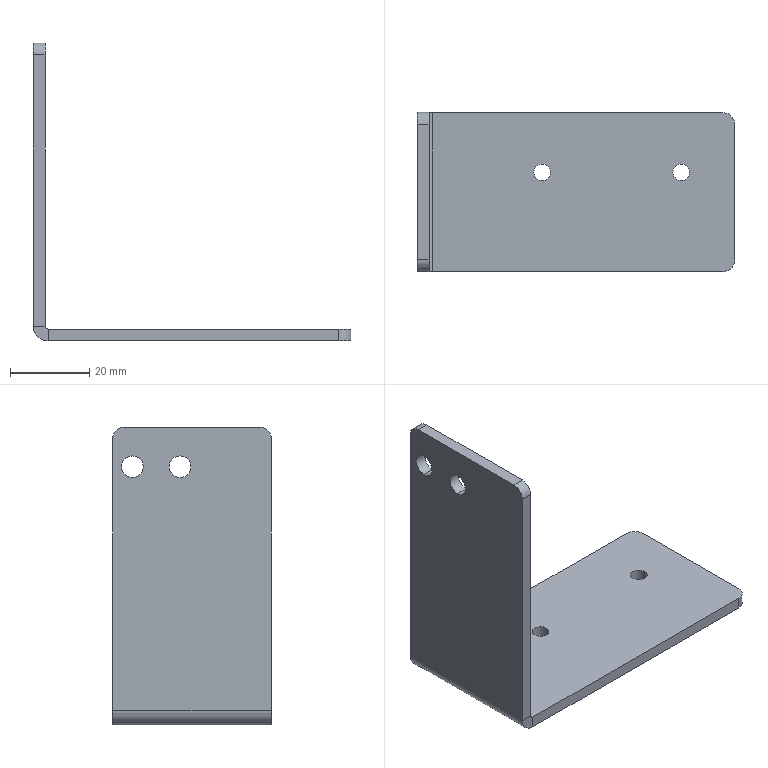Part | SolidWorks | features HoleWzd 2, Fillet 1, FlatPattern 1, SMBaseFlange 1, SheetMetal 1 | 1 solid | 26 faces | box 80 x 40 x 75 mm | volume 17875 mm3 | cylinder 14 | plane 12 | commonest cylinder face diameters 4.2 x4 5.5 x4 6 x4 1.5 x1 7.5 x1
STEP:
#1=CARTESIAN_POINT('',(3.,35.,-12.75));
#2=VERTEX_POINT('',#1);
#3=CARTESIAN_POINT('',(3.,35.,-7.25));
#4=VERTEX_POINT('',#3);
#5=CARTESIAN_POINT('',(3.,35.,-10.));
#6=DIRECTION('',(-1.,0.,0.));
#7=DIRECTION('',(0.,0.,1.));
#8=AXIS2_PLACEMENT_3D('',#5,#6,#7);
#9=CIRCLE('',#8,2.75);
#10=EDGE_CURVE('',#2,#4,#9,.T.);
#11=ORIENTED_EDGE('',*,*,#10,.F.);
#12=CARTESIAN_POINT('',(0.,35.,-12.75));
#13=VERTEX_POINT('',#12);
#14=CARTESIAN_POINT('',(0.,35.,-12.75));
#15=DIRECTION('',(-1.,0.,0.));
#16=VECTOR('',#15,1000.);
#17=LINE('',#14,#16);
#18=EDGE_CURVE('',#2,#13,#17,.T.);
#19=ORIENTED_EDGE('',*,*,#18,.T.);
#20=CARTESIAN_POINT('',(0.,35.,-7.25));
#21=VERTEX_POINT('',#20);
#22=CARTESIAN_POINT('',(0.,35.,-10.));
#23=DIRECTION('',(-1.,0.,0.));
#24=DIRECTION('',(0.,0.,1.));
#25=AXIS2_PLACEMENT_3D('',#22,#23,#24);
#26=CIRCLE('',#25,2.75);
#27=EDGE_CURVE('',#13,#21,#26,.T.);
#28=ORIENTED_EDGE('',*,*,#27,.T.);
#29=CARTESIAN_POINT('',(0.,35.,-7.25));
#30=DIRECTION('',(-1.,0.,0.));
#31=VECTOR('',#30,1000.);
#32=LINE('',#29,#31);
#33=EDGE_CURVE('',#4,#21,#32,.T.);
#34=ORIENTED_EDGE('',*,*,#33,.F.);
#35=EDGE_LOOP('',(#11,#19,#28,#34));
#36=FACE_OUTER_BOUND('',#35,.T.);
#37=CARTESIAN_POINT('',(0.,35.,-10.));
#38=DIRECTION('',(-1.,0.,0.));
#39=DIRECTION('',(0.,0.,1.));
#40=AXIS2_PLACEMENT_3D('',#37,#38,#39);
#41=CYLINDRICAL_SURFACE('',#40,2.75);
#42=ADVANCED_FACE('',(#36),#41,.F.);
#43=CARTESIAN_POINT('',(3.,23.,-12.75));
#44=VERTEX_POINT('',#43);
#45=CARTESIAN_POINT('',(3.,23.,-7.25));
#46=VERTEX_POINT('',#45);
#47=CARTESIAN_POINT('',(3.,23.,-10.));
#48=DIRECTION('',(-1.,0.,0.));
#49=DIRECTION('',(0.,0.,1.));
#50=AXIS2_PLACEMENT_3D('',#47,#48,#49);
#51=CIRCLE('',#50,2.75);
#52=EDGE_CURVE('',#44,#46,#51,.T.);
#53=ORIENTED_EDGE('',*,*,#52,.F.);
#54=CARTESIAN_POINT('',(0.,23.,-12.75));
#55=VERTEX_POINT('',#54);
#56=CARTESIAN_POINT('',(0.,23.,-12.75));
#57=DIRECTION('',(-1.,0.,0.));
#58=VECTOR('',#57,1000.);
#59=LINE('',#56,#58);
#60=EDGE_CURVE('',#44,#55,#59,.T.);
#61=ORIENTED_EDGE('',*,*,#60,.T.);
#62=CARTESIAN_POINT('',(0.,23.,-7.25));
#63=VERTEX_POINT('',#62);
#64=CARTESIAN_POINT('',(0.,23.,-10.));
#65=DIRECTION('',(-1.,0.,0.));
#66=DIRECTION('',(0.,0.,1.));
#67=AXIS2_PLACEMENT_3D('',#64,#65,#66);
#68=CIRCLE('',#67,2.75);
#69=EDGE_CURVE('',#55,#63,#68,.T.);
#70=ORIENTED_EDGE('',*,*,#69,.T.);
#71=CARTESIAN_POINT('',(0.,23.,-7.25));
#72=DIRECTION('',(-1.,0.,0.));
#73=VECTOR('',#72,1000.);
#74=LINE('',#71,#73);
#75=EDGE_CURVE('',#46,#63,#74,.T.);
#76=ORIENTED_EDGE('',*,*,#75,.F.);
#77=EDGE_LOOP('',(#53,#61,#70,#76));
#78=FACE_OUTER_BOUND('',#77,.T.);
#79=CARTESIAN_POINT('',(0.,23.,-10.));
#80=DIRECTION('',(-1.,0.,0.));
#81=DIRECTION('',(0.,0.,1.));
#82=AXIS2_PLACEMENT_3D('',#79,#80,#81);
#83=CYLINDRICAL_SURFACE('',#82,2.75);
#84=ADVANCED_FACE('',(#78),#83,.F.);
#85=CARTESIAN_POINT('',(68.6,25.,-72.));
#86=VERTEX_POINT('',#85);
#87=CARTESIAN_POINT('',(64.4,25.,-72.));
#88=VERTEX_POINT('',#87);
#89=CARTESIAN_POINT('',(66.5,25.,-72.));
#90=DIRECTION('',(0.,0.,-1.));
#91=DIRECTION('',(-1.,0.,0.));
#92=AXIS2_PLACEMENT_3D('',#89,#90,#91);
#93=CIRCLE('',#92,2.1);
#94=EDGE_CURVE('',#86,#88,#93,.T.);
#95=ORIENTED_EDGE('',*,*,#94,.F.);
#96=CARTESIAN_POINT('',(68.6,25.,-75.));
#97=VERTEX_POINT('',#96);
#98=CARTESIAN_POINT('',(68.6,25.,-75.));
#99=DIRECTION('',(0.,0.,-1.));
#100=VECTOR('',#99,1000.);
#101=LINE('',#98,#100);
#102=EDGE_CURVE('',#86,#97,#101,.T.);
#103=ORIENTED_EDGE('',*,*,#102,.T.);
#104=CARTESIAN_POINT('',(64.4,25.,-75.));
#105=VERTEX_POINT('',#104);
#106=CARTESIAN_POINT('',(66.5,25.,-75.));
#107=DIRECTION('',(0.,0.,-1.));
#108=DIRECTION('',(-1.,0.,0.));
#109=AXIS2_PLACEMENT_3D('',#106,#107,#108);
#110=CIRCLE('',#109,2.1);
#111=EDGE_CURVE('',#97,#105,#110,.T.);
#112=ORIENTED_EDGE('',*,*,#111,.T.);
#113=CARTESIAN_POINT('',(64.4,25.,-75.));
#114=DIRECTION('',(0.,0.,-1.));
#115=VECTOR('',#114,1000.);
#116=LINE('',#113,#115);
#117=EDGE_CURVE('',#88,#105,#116,.T.);
#118=ORIENTED_EDGE('',*,*,#117,.F.);
#119=EDGE_LOOP('',(#95,#103,#112,#118));
#120=FACE_OUTER_BOUND('',#119,.T.);
#121=CARTESIAN_POINT('',(66.5,25.,-75.));
#122=DIRECTION('',(0.,0.,-1.));
#123=DIRECTION('',(-1.,0.,0.));
#124=AXIS2_PLACEMENT_3D('',#121,#122,#123);
#125=CYLINDRICAL_SURFACE('',#124,2.1);
#126=ADVANCED_FACE('',(#120),#125,.F.);
#127=CARTESIAN_POINT('',(33.6,25.,-72.));
#128=VERTEX_POINT('',#127);
#129=CARTESIAN_POINT('',(29.4,25.,-72.));
#130=VERTEX_POINT('',#129);
#131=CARTESIAN_POINT('',(31.5,25.,-72.));
#132=DIRECTION('',(0.,0.,-1.));
#133=DIRECTION('',(-1.,0.,0.));
#134=AXIS2_PLACEMENT_3D('',#131,#132,#133);
#135=CIRCLE('',#134,2.1);
#136=EDGE_CURVE('',#128,#130,#135,.T.);
#137=ORIENTED_EDGE('',*,*,#136,.F.);
#138=CARTESIAN_POINT('',(33.6,25.,-75.));
#139=VERTEX_POINT('',#138);
#140=CARTESIAN_POINT('',(33.6,25.,-75.));
#141=DIRECTION('',(0.,0.,-1.));
#142=VECTOR('',#141,1000.);
#143=LINE('',#140,#142);
#144=EDGE_CURVE('',#128,#139,#143,.T.);
#145=ORIENTED_EDGE('',*,*,#144,.T.);
#146=CARTESIAN_POINT('',(29.4,25.,-75.));
#147=VERTEX_POINT('',#146);
#148=CARTESIAN_POINT('',(31.5,25.,-75.));
#149=DIRECTION('',(0.,0.,-1.));
#150=DIRECTION('',(-1.,0.,0.));
#151=AXIS2_PLACEMENT_3D('',#148,#149,#150);
#152=CIRCLE('',#151,2.1);
#153=EDGE_CURVE('',#139,#147,#152,.T.);
#154=ORIENTED_EDGE('',*,*,#153,.T.);
#155=CARTESIAN_POINT('',(29.4,25.,-75.));
#156=DIRECTION('',(0.,0.,-1.));
#157=VECTOR('',#156,1000.);
#158=LINE('',#155,#157);
#159=EDGE_CURVE('',#130,#147,#158,.T.);
#160=ORIENTED_EDGE('',*,*,#159,.F.);
#161=EDGE_LOOP('',(#137,#145,#154,#160));
#162=FACE_OUTER_BOUND('',#161,.T.);
#163=CARTESIAN_POINT('',(31.5,25.,-75.));
#164=DIRECTION('',(0.,0.,-1.));
#165=DIRECTION('',(-1.,0.,0.));
#166=AXIS2_PLACEMENT_3D('',#163,#164,#165);
#167=CYLINDRICAL_SURFACE('',#166,2.1);
#168=ADVANCED_FACE('',(#162),#167,.F.);
#169=CARTESIAN_POINT('',(3.75,40.,-75.));
#170=VERTEX_POINT('',#169);
#171=CARTESIAN_POINT('',(3.75,40.,-72.));
#172=VERTEX_POINT('',#171);
#173=CARTESIAN_POINT('',(3.75,40.,-75.));
#174=DIRECTION('',(0.,0.,1.));
#175=VECTOR('',#174,1000.);
#176=LINE('',#173,#175);
#177=EDGE_CURVE('',#170,#172,#176,.T.);
#178=ORIENTED_EDGE('',*,*,#177,.F.);
#179=CARTESIAN_POINT('',(0.,40.,-71.25));
#180=VERTEX_POINT('',#179);
#181=CARTESIAN_POINT('',(3.75,40.,-71.25));
#182=DIRECTION('',(0.,-1.,0.));
#183=DIRECTION('',(0.,0.,1.));
#184=AXIS2_PLACEMENT_3D('',#181,#182,#183);
#185=CIRCLE('',#184,3.75);
#186=EDGE_CURVE('',#180,#170,#185,.T.);
#187=ORIENTED_EDGE('',*,*,#186,.F.);
#188=CARTESIAN_POINT('',(3.,40.,-71.25));
#189=VERTEX_POINT('',#188);
#190=CARTESIAN_POINT('',(3.,40.,-71.25));
#191=DIRECTION('',(-1.,0.,0.));
#192=VECTOR('',#191,1000.);
#193=LINE('',#190,#192);
#194=EDGE_CURVE('',#189,#180,#193,.T.);
#195=ORIENTED_EDGE('',*,*,#194,.F.);
#196=CARTESIAN_POINT('',(3.75,40.,-71.25));
#197=DIRECTION('',(0.,-1.,0.));
#198=DIRECTION('',(1.,0.,0.));
#199=AXIS2_PLACEMENT_3D('',#196,#197,#198);
#200=CIRCLE('',#199,0.75);
#201=EDGE_CURVE('',#189,#172,#200,.T.);
#202=ORIENTED_EDGE('',*,*,#201,.T.);
#203=EDGE_LOOP('',(#178,#187,#195,#202));
#204=FACE_OUTER_BOUND('',#203,.T.);
#205=CARTESIAN_POINT('',(3.75,40.,-75.));
#206=DIRECTION('',(0.,1.,0.));
#207=DIRECTION('',(0.,0.,1.));
#208=AXIS2_PLACEMENT_3D('',#205,#206,#207);
#209=PLANE('',#208);
#210=ADVANCED_FACE('',(#204),#209,.T.);
#211=CARTESIAN_POINT('',(77.,40.,-72.));
#212=VERTEX_POINT('',#211);
#213=CARTESIAN_POINT('',(0.,40.,-72.));
#214=DIRECTION('',(1.,0.,0.));
#215=VECTOR('',#214,1000.);
#216=LINE('',#213,#215);
#217=EDGE_CURVE('',#172,#212,#216,.T.);
#218=ORIENTED_EDGE('',*,*,#217,.T.);
#219=CARTESIAN_POINT('',(77.,40.,-75.));
#220=VERTEX_POINT('',#219);
#221=CARTESIAN_POINT('',(77.,40.,-71.25));
#222=DIRECTION('',(0.,0.,-1.));
#223=VECTOR('',#222,1000.);
#224=LINE('',#221,#223);
#225=EDGE_CURVE('',#212,#220,#224,.T.);
#226=ORIENTED_EDGE('',*,*,#225,.T.);
#227=CARTESIAN_POINT('',(0.,40.,-75.));
#228=DIRECTION('',(1.,0.,0.));
#229=VECTOR('',#228,1000.);
#230=LINE('',#227,#229);
#231=EDGE_CURVE('',#170,#220,#230,.T.);
#232=ORIENTED_EDGE('',*,*,#231,.F.);
#233=ORIENTED_EDGE('',*,*,#177,.T.);
#234=EDGE_LOOP('',(#218,#226,#232,#233));
#235=FACE_OUTER_BOUND('',#234,.T.);
#236=CARTESIAN_POINT('',(3.,40.,-71.25));
#237=DIRECTION('',(0.,1.,0.));
#238=DIRECTION('',(0.,0.,1.));
#239=AXIS2_PLACEMENT_3D('',#236,#237,#238);
#240=PLANE('',#239);
#241=ADVANCED_FACE('',(#235),#240,.T.);
#242=CARTESIAN_POINT('',(0.,0.,-71.25));
#243=VERTEX_POINT('',#242);
#244=CARTESIAN_POINT('',(3.,0.,-71.25));
#245=VERTEX_POINT('',#244);
#246=CARTESIAN_POINT('',(0.,0.,-71.25));
#247=DIRECTION('',(1.,0.,0.));
#248=VECTOR('',#247,1000.);
#249=LINE('',#246,#248);
#250=EDGE_CURVE('',#243,#245,#249,.T.);
#251=ORIENTED_EDGE('',*,*,#250,.F.);
#252=CARTESIAN_POINT('',(3.75,0.,-75.));
#253=VERTEX_POINT('',#252);
#254=CARTESIAN_POINT('',(3.75,0.,-71.25));
#255=DIRECTION('',(0.,-1.,0.));
#256=DIRECTION('',(0.,0.,1.));
#257=AXIS2_PLACEMENT_3D('',#254,#255,#256);
#258=CIRCLE('',#257,3.75);
#259=EDGE_CURVE('',#243,#253,#258,.T.);
#260=ORIENTED_EDGE('',*,*,#259,.T.);
#261=CARTESIAN_POINT('',(3.75,0.,-72.));
#262=VERTEX_POINT('',#261);
#263=CARTESIAN_POINT('',(3.75,0.,-72.));
#264=DIRECTION('',(0.,0.,-1.));
#265=VECTOR('',#264,1000.);
#266=LINE('',#263,#265);
#267=EDGE_CURVE('',#262,#253,#266,.T.);
#268=ORIENTED_EDGE('',*,*,#267,.F.);
#269=CARTESIAN_POINT('',(3.75,0.,-71.25));
#270=DIRECTION('',(0.,-1.,0.));
#271=DIRECTION('',(1.,0.,0.));
#272=AXIS2_PLACEMENT_3D('',#269,#270,#271);
#273=CIRCLE('',#272,0.75);
#274=EDGE_CURVE('',#245,#262,#273,.T.);
#275=ORIENTED_EDGE('',*,*,#274,.F.);
#276=EDGE_LOOP('',(#251,#260,#268,#275));
#277=FACE_OUTER_BOUND('',#276,.T.);
#278=CARTESIAN_POINT('',(0.,0.,-71.25));
#279=DIRECTION('',(0.,-1.,0.));
#280=DIRECTION('',(0.,0.,-1.));
#281=AXIS2_PLACEMENT_3D('',#278,#279,#280);
#282=PLANE('',#281);
#283=ADVANCED_FACE('',(#277),#282,.T.);
#284=CARTESIAN_POINT('',(3.,0.,-3.));
#285=VERTEX_POINT('',#284);
#286=CARTESIAN_POINT('',(3.,0.,0.));
#287=DIRECTION('',(0.,0.,-1.));
#288=VECTOR('',#287,1000.);
#289=LINE('',#286,#288);
#290=EDGE_CURVE('',#285,#245,#289,.T.);
#291=ORIENTED_EDGE('',*,*,#290,.F.);
#292=CARTESIAN_POINT('',(0.,0.,-3.));
#293=VERTEX_POINT('',#292);
#294=CARTESIAN_POINT('',(3.75,0.,-3.));
#295=DIRECTION('',(-1.,0.,0.));
#296=VECTOR('',#295,1000.);
#297=LINE('',#294,#296);
#298=EDGE_CURVE('',#285,#293,#297,.T.);
#299=ORIENTED_EDGE('',*,*,#298,.T.);
#300=CARTESIAN_POINT('',(0.,0.,0.));
#301=DIRECTION('',(0.,0.,-1.));
#302=VECTOR('',#301,1000.);
#303=LINE('',#300,#302);
#304=EDGE_CURVE('',#293,#243,#303,.T.);
#305=ORIENTED_EDGE('',*,*,#304,.T.);
#306=ORIENTED_EDGE('',*,*,#250,.T.);
#307=EDGE_LOOP('',(#291,#299,#305,#306));
#308=FACE_OUTER_BOUND('',#307,.T.);
#309=CARTESIAN_POINT('',(3.75,0.,-72.));
#310=DIRECTION('',(0.,-1.,0.));
#311=DIRECTION('',(0.,0.,-1.));
#312=AXIS2_PLACEMENT_3D('',#309,#310,#311);
#313=PLANE('',#312);
#314=ADVANCED_FACE('',(#308),#313,.T.);
#315=CARTESIAN_POINT('',(66.5,25.,-72.));
#316=DIRECTION('',(0.,0.,-1.));
#317=DIRECTION('',(-1.,0.,0.));
#318=AXIS2_PLACEMENT_3D('',#315,#316,#317);
#319=CIRCLE('',#318,2.1);
#320=EDGE_CURVE('',#88,#86,#319,.T.);
#321=ORIENTED_EDGE('',*,*,#320,.T.);
#322=ORIENTED_EDGE('',*,*,#94,.T.);
#323=EDGE_LOOP('',(#321,#322));
#324=FACE_BOUND('',#323,.T.);
#325=CARTESIAN_POINT('',(31.5,25.,-72.));
#326=DIRECTION('',(0.,0.,-1.));
#327=DIRECTION('',(-1.,0.,0.));
#328=AXIS2_PLACEMENT_3D('',#325,#326,#327);
#329=CIRCLE('',#328,2.1);
#330=EDGE_CURVE('',#130,#128,#329,.T.);
#331=ORIENTED_EDGE('',*,*,#330,.T.);
#332=ORIENTED_EDGE('',*,*,#136,.T.);
#333=EDGE_LOOP('',(#331,#332));
#334=FACE_BOUND('',#333,.T.);
#335=CARTESIAN_POINT('',(80.,37.,-72.));
#336=VERTEX_POINT('',#335);
#337=CARTESIAN_POINT('',(80.,3.,-72.));
#338=VERTEX_POINT('',#337);
#339=CARTESIAN_POINT('',(80.,40.,-72.));
#340=DIRECTION('',(0.,-1.,0.));
#341=VECTOR('',#340,1000.);
#342=LINE('',#339,#341);
#343=EDGE_CURVE('',#336,#338,#342,.T.);
#344=ORIENTED_EDGE('',*,*,#343,.F.);
#345=CARTESIAN_POINT('',(77.,37.,-72.));
#346=DIRECTION('',(0.,0.,1.));
#347=DIRECTION('',(-1.,0.,0.));
#348=AXIS2_PLACEMENT_3D('',#345,#346,#347);
#349=CIRCLE('',#348,3.);
#350=EDGE_CURVE('',#336,#212,#349,.T.);
#351=ORIENTED_EDGE('',*,*,#350,.T.);
#352=ORIENTED_EDGE('',*,*,#217,.F.);
#353=CARTESIAN_POINT('',(3.75,40.,-72.));
#354=DIRECTION('',(0.,-1.,0.));
#355=VECTOR('',#354,1000.);
#356=LINE('',#353,#355);
#357=EDGE_CURVE('',#172,#262,#356,.T.);
#358=ORIENTED_EDGE('',*,*,#357,.T.);
#359=CARTESIAN_POINT('',(77.,0.,-72.));
#360=VERTEX_POINT('',#359);
#361=CARTESIAN_POINT('',(0.,0.,-72.));
#362=DIRECTION('',(1.,0.,0.));
#363=VECTOR('',#362,1000.);
#364=LINE('',#361,#363);
#365=EDGE_CURVE('',#262,#360,#364,.T.);
#366=ORIENTED_EDGE('',*,*,#365,.T.);
#367=CARTESIAN_POINT('',(77.,3.,-72.));
#368=DIRECTION('',(0.,0.,1.));
#369=DIRECTION('',(-1.,0.,0.));
#370=AXIS2_PLACEMENT_3D('',#367,#368,#369);
#371=CIRCLE('',#370,3.);
#372=EDGE_CURVE('',#360,#338,#371,.T.);
#373=ORIENTED_EDGE('',*,*,#372,.T.);
#374=EDGE_LOOP('',(#344,#351,#352,#358,#366,#373));
#375=FACE_OUTER_BOUND('',#374,.T.);
#376=CARTESIAN_POINT('',(0.,40.,-72.));
#377=DIRECTION('',(0.,0.,-1.));
#378=DIRECTION('',(-1.,0.,0.));
#379=AXIS2_PLACEMENT_3D('',#376,#377,#378);
#380=PLANE('',#379);
#381=ADVANCED_FACE('',(#324,#334,#375),#380,.F.);
#382=CARTESIAN_POINT('',(80.,37.,-75.));
#383=VERTEX_POINT('',#382);
#384=CARTESIAN_POINT('',(80.,3.,-75.));
#385=VERTEX_POINT('',#384);
#386=CARTESIAN_POINT('',(80.,40.,-75.));
#387=DIRECTION('',(0.,-1.,0.));
#388=VECTOR('',#387,1000.);
#389=LINE('',#386,#388);
#390=EDGE_CURVE('',#383,#385,#389,.T.);
#391=ORIENTED_EDGE('',*,*,#390,.F.);
#392=CARTESIAN_POINT('',(80.,37.,-75.));
#393=DIRECTION('',(0.,0.,1.));
#394=VECTOR('',#393,1000.);
#395=LINE('',#392,#394);
#396=EDGE_CURVE('',#383,#336,#395,.T.);
#397=ORIENTED_EDGE('',*,*,#396,.T.);
#398=ORIENTED_EDGE('',*,*,#343,.T.);
#399=CARTESIAN_POINT('',(80.,3.,-75.));
#400=DIRECTION('',(0.,0.,-1.));
#401=VECTOR('',#400,1000.);
#402=LINE('',#399,#401);
#403=EDGE_CURVE('',#338,#385,#402,.T.);
#404=ORIENTED_EDGE('',*,*,#403,.T.);
#405=EDGE_LOOP('',(#391,#397,#398,#404));
#406=FACE_OUTER_BOUND('',#405,.T.);
#407=CARTESIAN_POINT('',(80.,40.,-75.));
#408=DIRECTION('',(1.,0.,0.));
#409=DIRECTION('',(0.,0.,-1.));
#410=AXIS2_PLACEMENT_3D('',#407,#408,#409);
#411=PLANE('',#410);
#412=ADVANCED_FACE('',(#406),#411,.T.);
#413=CARTESIAN_POINT('',(66.5,25.,-75.));
#414=DIRECTION('',(0.,0.,-1.));
#415=DIRECTION('',(-1.,0.,0.));
#416=AXIS2_PLACEMENT_3D('',#413,#414,#415);
#417=CIRCLE('',#416,2.1);
#418=EDGE_CURVE('',#105,#97,#417,.T.);
#419=ORIENTED_EDGE('',*,*,#418,.F.);
#420=ORIENTED_EDGE('',*,*,#111,.F.);
#421=EDGE_LOOP('',(#419,#420));
#422=FACE_BOUND('',#421,.T.);
#423=CARTESIAN_POINT('',(31.5,25.,-75.));
#424=DIRECTION('',(0.,0.,-1.));
#425=DIRECTION('',(-1.,0.,0.));
#426=AXIS2_PLACEMENT_3D('',#423,#424,#425);
#427=CIRCLE('',#426,2.1);
#428=EDGE_CURVE('',#147,#139,#427,.T.);
#429=ORIENTED_EDGE('',*,*,#428,.F.);
#430=ORIENTED_EDGE('',*,*,#153,.F.);
#431=EDGE_LOOP('',(#429,#430));
#432=FACE_BOUND('',#431,.T.);
#433=ORIENTED_EDGE('',*,*,#231,.T.);
#434=CARTESIAN_POINT('',(77.,37.,-75.));
#435=DIRECTION('',(0.,0.,-1.));
#436=DIRECTION('',(-1.,0.,0.));
#437=AXIS2_PLACEMENT_3D('',#434,#435,#436);
#438=CIRCLE('',#437,3.);
#439=EDGE_CURVE('',#220,#383,#438,.T.);
#440=ORIENTED_EDGE('',*,*,#439,.T.);
#441=ORIENTED_EDGE('',*,*,#390,.T.);
#442=CARTESIAN_POINT('',(77.,0.,-75.));
#443=VERTEX_POINT('',#442);
#444=CARTESIAN_POINT('',(77.,3.,-75.));
#445=DIRECTION('',(0.,0.,-1.));
#446=DIRECTION('',(-1.,0.,0.));
#447=AXIS2_PLACEMENT_3D('',#444,#445,#446);
#448=CIRCLE('',#447,3.);
#449=EDGE_CURVE('',#385,#443,#448,.T.);
#450=ORIENTED_EDGE('',*,*,#449,.T.);
#451=CARTESIAN_POINT('',(0.,0.,-75.));
#452=DIRECTION('',(1.,0.,0.));
#453=VECTOR('',#452,1000.);
#454=LINE('',#451,#453);
#455=EDGE_CURVE('',#253,#443,#454,.T.);
#456=ORIENTED_EDGE('',*,*,#455,.F.);
#457=CARTESIAN_POINT('',(3.75,40.,-75.));
#458=DIRECTION('',(0.,-1.,0.));
#459=VECTOR('',#458,1000.);
#460=LINE('',#457,#459);
#461=EDGE_CURVE('',#170,#253,#460,.T.);
#462=ORIENTED_EDGE('',*,*,#461,.F.);
#463=EDGE_LOOP('',(#433,#440,#441,#450,#456,#462));
#464=FACE_OUTER_BOUND('',#463,.T.);
#465=CARTESIAN_POINT('',(0.,40.,-75.));
#466=DIRECTION('',(0.,0.,-1.));
#467=DIRECTION('',(-1.,0.,0.));
#468=AXIS2_PLACEMENT_3D('',#465,#466,#467);
#469=PLANE('',#468);
#470=ADVANCED_FACE('',(#422,#432,#464),#469,.T.);
#471=ORIENTED_EDGE('',*,*,#259,.F.);
#472=CARTESIAN_POINT('',(0.,40.,-71.25));
#473=DIRECTION('',(0.,-1.,0.));
#474=VECTOR('',#473,1000.);
#475=LINE('',#472,#474);
#476=EDGE_CURVE('',#180,#243,#475,.T.);
#477=ORIENTED_EDGE('',*,*,#476,.F.);
#478=ORIENTED_EDGE('',*,*,#186,.T.);
#479=ORIENTED_EDGE('',*,*,#461,.T.);
#480=EDGE_LOOP('',(#471,#477,#478,#479));
#481=FACE_OUTER_BOUND('',#480,.T.);
#482=CARTESIAN_POINT('',(3.75,40.,-71.25));
#483=DIRECTION('',(0.,-1.,0.));
#484=DIRECTION('',(0.,0.,-1.));
#485=AXIS2_PLACEMENT_3D('',#482,#483,#484);
#486=CYLINDRICAL_SURFACE('',#485,3.75);
#487=ADVANCED_FACE('',(#481),#486,.T.);
#488=CARTESIAN_POINT('',(0.,35.,-10.));
#489=DIRECTION('',(-1.,0.,0.));
#490=DIRECTION('',(0.,0.,1.));
#491=AXIS2_PLACEMENT_3D('',#488,#489,#490);
#492=CIRCLE('',#491,2.75);
#493=EDGE_CURVE('',#21,#13,#492,.T.);
#494=ORIENTED_EDGE('',*,*,#493,.F.);
#495=ORIENTED_EDGE('',*,*,#27,.F.);
#496=EDGE_LOOP('',(#494,#495));
#497=FACE_BOUND('',#496,.T.);
#498=CARTESIAN_POINT('',(0.,23.,-10.));
#499=DIRECTION('',(-1.,0.,0.));
#500=DIRECTION('',(0.,0.,1.));
#501=AXIS2_PLACEMENT_3D('',#498,#499,#500);
#502=CIRCLE('',#501,2.75);
#503=EDGE_CURVE('',#63,#55,#502,.T.);
#504=ORIENTED_EDGE('',*,*,#503,.F.);
#505=ORIENTED_EDGE('',*,*,#69,.F.);
#506=EDGE_LOOP('',(#504,#505));
#507=FACE_BOUND('',#506,.T.);
#508=ORIENTED_EDGE('',*,*,#304,.F.);
#509=CARTESIAN_POINT('',(0.,3.,0.));
#510=VERTEX_POINT('',#509);
#511=CARTESIAN_POINT('',(0.,3.,-3.));
#512=DIRECTION('',(-1.,0.,0.));
#513=DIRECTION('',(0.,0.,1.));
#514=AXIS2_PLACEMENT_3D('',#511,#512,#513);
#515=CIRCLE('',#514,3.);
#516=EDGE_CURVE('',#293,#510,#515,.T.);
#517=ORIENTED_EDGE('',*,*,#516,.T.);
#518=CARTESIAN_POINT('',(0.,37.,0.));
#519=VERTEX_POINT('',#518);
#520=CARTESIAN_POINT('',(0.,40.,0.));
#521=DIRECTION('',(0.,-1.,0.));
#522=VECTOR('',#521,1000.);
#523=LINE('',#520,#522);
#524=EDGE_CURVE('',#519,#510,#523,.T.);
#525=ORIENTED_EDGE('',*,*,#524,.F.);
#526=CARTESIAN_POINT('',(0.,40.,-3.));
#527=VERTEX_POINT('',#526);
#528=CARTESIAN_POINT('',(0.,37.,-3.));
#529=DIRECTION('',(-1.,0.,0.));
#530=DIRECTION('',(0.,0.,1.));
#531=AXIS2_PLACEMENT_3D('',#528,#529,#530);
#532=CIRCLE('',#531,3.);
#533=EDGE_CURVE('',#519,#527,#532,.T.);
#534=ORIENTED_EDGE('',*,*,#533,.T.);
#535=CARTESIAN_POINT('',(0.,40.,0.));
#536=DIRECTION('',(0.,0.,-1.));
#537=VECTOR('',#536,1000.);
#538=LINE('',#535,#537);
#539=EDGE_CURVE('',#527,#180,#538,.T.);
#540=ORIENTED_EDGE('',*,*,#539,.T.);
#541=ORIENTED_EDGE('',*,*,#476,.T.);
#542=EDGE_LOOP('',(#508,#517,#525,#534,#540,#541));
#543=FACE_OUTER_BOUND('',#542,.T.);
#544=CARTESIAN_POINT('',(0.,40.,0.));
#545=DIRECTION('',(-1.,0.,0.));
#546=DIRECTION('',(0.,0.,1.));
#547=AXIS2_PLACEMENT_3D('',#544,#545,#546);
#548=PLANE('',#547);
#549=ADVANCED_FACE('',(#497,#507,#543),#548,.T.);
#550=ORIENTED_EDGE('',*,*,#524,.T.);
#551=CARTESIAN_POINT('',(3.,3.,0.));
#552=VERTEX_POINT('',#551);
#553=CARTESIAN_POINT('',(3.,3.,0.));
#554=DIRECTION('',(1.,0.,0.));
#555=VECTOR('',#554,1000.);
#556=LINE('',#553,#555);
#557=EDGE_CURVE('',#510,#552,#556,.T.);
#558=ORIENTED_EDGE('',*,*,#557,.T.);
#559=CARTESIAN_POINT('',(3.,37.,0.));
#560=VERTEX_POINT('',#559);
#561=CARTESIAN_POINT('',(3.,40.,0.));
#562=DIRECTION('',(0.,-1.,0.));
#563=VECTOR('',#562,1000.);
#564=LINE('',#561,#563);
#565=EDGE_CURVE('',#560,#552,#564,.T.);
#566=ORIENTED_EDGE('',*,*,#565,.F.);
#567=CARTESIAN_POINT('',(3.,37.,0.));
#568=DIRECTION('',(-1.,0.,0.));
#569=VECTOR('',#568,1000.);
#570=LINE('',#567,#569);
#571=EDGE_CURVE('',#560,#519,#570,.T.);
#572=ORIENTED_EDGE('',*,*,#571,.T.);
#573=EDGE_LOOP('',(#550,#558,#566,#572));
#574=FACE_OUTER_BOUND('',#573,.T.);
#575=CARTESIAN_POINT('',(3.,40.,0.));
#576=DIRECTION('',(0.,0.,1.));
#577=DIRECTION('',(1.,0.,0.));
#578=AXIS2_PLACEMENT_3D('',#575,#576,#577);
#579=PLANE('',#578);
#580=ADVANCED_FACE('',(#574),#579,.T.);
#581=CARTESIAN_POINT('',(3.,35.,-10.));
#582=DIRECTION('',(-1.,0.,0.));
#583=DIRECTION('',(0.,0.,1.));
#584=AXIS2_PLACEMENT_3D('',#581,#582,#583);
#585=CIRCLE('',#584,2.75);
#586=EDGE_CURVE('',#4,#2,#585,.T.);
#587=ORIENTED_EDGE('',*,*,#586,.T.);
#588=ORIENTED_EDGE('',*,*,#10,.T.);
#589=EDGE_LOOP('',(#587,#588));
#590=FACE_BOUND('',#589,.T.);
#591=CARTESIAN_POINT('',(3.,23.,-10.));
#592=DIRECTION('',(-1.,0.,0.));
#593=DIRECTION('',(0.,0.,1.));
#594=AXIS2_PLACEMENT_3D('',#591,#592,#593);
#595=CIRCLE('',#594,2.75);
#596=EDGE_CURVE('',#46,#44,#595,.T.);
#597=ORIENTED_EDGE('',*,*,#596,.T.);
#598=ORIENTED_EDGE('',*,*,#52,.T.);
#599=EDGE_LOOP('',(#597,#598));
#600=FACE_BOUND('',#599,.T.);
#601=ORIENTED_EDGE('',*,*,#565,.T.);
#602=CARTESIAN_POINT('',(3.,3.,-3.));
#603=DIRECTION('',(1.,0.,0.));
#604=DIRECTION('',(0.,0.,1.));
#605=AXIS2_PLACEMENT_3D('',#602,#603,#604);
#606=CIRCLE('',#605,3.);
#607=EDGE_CURVE('',#552,#285,#606,.T.);
#608=ORIENTED_EDGE('',*,*,#607,.T.);
#609=ORIENTED_EDGE('',*,*,#290,.T.);
#610=CARTESIAN_POINT('',(3.,40.,-71.25));
#611=DIRECTION('',(0.,-1.,0.));
#612=VECTOR('',#611,1000.);
#613=LINE('',#610,#612);
#614=EDGE_CURVE('',#189,#245,#613,.T.);
#615=ORIENTED_EDGE('',*,*,#614,.F.);
#616=CARTESIAN_POINT('',(3.,40.,-3.));
#617=VERTEX_POINT('',#616);
#618=CARTESIAN_POINT('',(3.,40.,0.));
#619=DIRECTION('',(0.,0.,-1.));
#620=VECTOR('',#619,1000.);
#621=LINE('',#618,#620);
#622=EDGE_CURVE('',#617,#189,#621,.T.);
#623=ORIENTED_EDGE('',*,*,#622,.F.);
#624=CARTESIAN_POINT('',(3.,37.,-3.));
#625=DIRECTION('',(1.,0.,0.));
#626=DIRECTION('',(0.,0.,1.));
#627=AXIS2_PLACEMENT_3D('',#624,#625,#626);
#628=CIRCLE('',#627,3.);
#629=EDGE_CURVE('',#617,#560,#628,.T.);
#630=ORIENTED_EDGE('',*,*,#629,.T.);
#631=EDGE_LOOP('',(#601,#608,#609,#615,#623,#630));
#632=FACE_OUTER_BOUND('',#631,.T.);
#633=CARTESIAN_POINT('',(3.,40.,0.));
#634=DIRECTION('',(-1.,0.,0.));
#635=DIRECTION('',(0.,0.,1.));
#636=AXIS2_PLACEMENT_3D('',#633,#634,#635);
#637=PLANE('',#636);
#638=ADVANCED_FACE('',(#590,#600,#632),#637,.F.);
#639=ORIENTED_EDGE('',*,*,#274,.T.);
#640=ORIENTED_EDGE('',*,*,#357,.F.);
#641=ORIENTED_EDGE('',*,*,#201,.F.);
#642=ORIENTED_EDGE('',*,*,#614,.T.);
#643=EDGE_LOOP('',(#639,#640,#641,#642));
#644=FACE_OUTER_BOUND('',#643,.T.);
#645=CARTESIAN_POINT('',(3.75,40.,-71.25));
#646=DIRECTION('',(0.,-1.,0.));
#647=DIRECTION('',(0.,0.,-1.));
#648=AXIS2_PLACEMENT_3D('',#645,#646,#647);
#649=CYLINDRICAL_SURFACE('',#648,0.75);
#650=ADVANCED_FACE('',(#644),#649,.F.);
#651=ORIENTED_EDGE('',*,*,#539,.F.);
#652=CARTESIAN_POINT('',(3.75,40.,-3.));
#653=DIRECTION('',(1.,0.,0.));
#654=VECTOR('',#653,1000.);
#655=LINE('',#652,#654);
#656=EDGE_CURVE('',#527,#617,#655,.T.);
#657=ORIENTED_EDGE('',*,*,#656,.T.);
#658=ORIENTED_EDGE('',*,*,#622,.T.);
#659=ORIENTED_EDGE('',*,*,#194,.T.);
#660=EDGE_LOOP('',(#651,#657,#658,#659));
#661=FACE_OUTER_BOUND('',#660,.T.);
#662=CARTESIAN_POINT('',(3.75,40.,-71.25));
#663=DIRECTION('',(0.,1.,0.));
#664=DIRECTION('',(1.,0.,0.));
#665=AXIS2_PLACEMENT_3D('',#662,#663,#664);
#666=PLANE('',#665);
#667=ADVANCED_FACE('',(#661),#666,.T.);
#668=ORIENTED_EDGE('',*,*,#455,.T.);
#669=CARTESIAN_POINT('',(77.,0.,-72.));
#670=DIRECTION('',(0.,0.,1.));
#671=VECTOR('',#670,1000.);
#672=LINE('',#669,#671);
#673=EDGE_CURVE('',#443,#360,#672,.T.);
#674=ORIENTED_EDGE('',*,*,#673,.T.);
#675=ORIENTED_EDGE('',*,*,#365,.F.);
#676=ORIENTED_EDGE('',*,*,#267,.T.);
#677=EDGE_LOOP('',(#668,#674,#675,#676));
#678=FACE_OUTER_BOUND('',#677,.T.);
#679=CARTESIAN_POINT('',(3.75,0.,-71.25));
#680=DIRECTION('',(0.,1.,0.));
#681=DIRECTION('',(1.,0.,0.));
#682=AXIS2_PLACEMENT_3D('',#679,#680,#681);
#683=PLANE('',#682);
#684=ADVANCED_FACE('',(#678),#683,.F.);
#685=ORIENTED_EDGE('',*,*,#439,.F.);
#686=ORIENTED_EDGE('',*,*,#225,.F.);
#687=ORIENTED_EDGE('',*,*,#350,.F.);
#688=ORIENTED_EDGE('',*,*,#396,.F.);
#689=EDGE_LOOP('',(#685,#686,#687,#688));
#690=FACE_OUTER_BOUND('',#689,.T.);
#691=CARTESIAN_POINT('',(77.,37.,-75.));
#692=DIRECTION('',(0.,0.,1.));
#693=DIRECTION('',(1.,0.,0.));
#694=AXIS2_PLACEMENT_3D('',#691,#692,#693);
#695=CYLINDRICAL_SURFACE('',#694,3.);
#696=ADVANCED_FACE('',(#690),#695,.T.);
#697=ORIENTED_EDGE('',*,*,#449,.F.);
#698=ORIENTED_EDGE('',*,*,#403,.F.);
#699=ORIENTED_EDGE('',*,*,#372,.F.);
#700=ORIENTED_EDGE('',*,*,#673,.F.);
#701=EDGE_LOOP('',(#697,#698,#699,#700));
#702=FACE_OUTER_BOUND('',#701,.T.);
#703=CARTESIAN_POINT('',(77.,3.,-71.25));
#704=DIRECTION('',(0.,0.,-1.));
#705=DIRECTION('',(-1.,0.,0.));
#706=AXIS2_PLACEMENT_3D('',#703,#704,#705);
#707=CYLINDRICAL_SURFACE('',#706,3.);
#708=ADVANCED_FACE('',(#702),#707,.T.);
#709=ORIENTED_EDGE('',*,*,#607,.F.);
#710=ORIENTED_EDGE('',*,*,#557,.F.);
#711=ORIENTED_EDGE('',*,*,#516,.F.);
#712=ORIENTED_EDGE('',*,*,#298,.F.);
#713=EDGE_LOOP('',(#709,#710,#711,#712));
#714=FACE_OUTER_BOUND('',#713,.T.);
#715=CARTESIAN_POINT('',(3.75,3.,-3.));
#716=DIRECTION('',(-1.,0.,0.));
#717=DIRECTION('',(0.,0.,1.));
#718=AXIS2_PLACEMENT_3D('',#715,#716,#717);
#719=CYLINDRICAL_SURFACE('',#718,3.);
#720=ADVANCED_FACE('',(#714),#719,.T.);
#721=ORIENTED_EDGE('',*,*,#629,.F.);
#722=ORIENTED_EDGE('',*,*,#656,.F.);
#723=ORIENTED_EDGE('',*,*,#533,.F.);
#724=ORIENTED_EDGE('',*,*,#571,.F.);
#725=EDGE_LOOP('',(#721,#722,#723,#724));
#726=FACE_OUTER_BOUND('',#725,.T.);
#727=CARTESIAN_POINT('',(3.,37.,-3.));
#728=DIRECTION('',(-1.,0.,0.));
#729=DIRECTION('',(0.,0.,1.));
#730=AXIS2_PLACEMENT_3D('',#727,#728,#729);
#731=CYLINDRICAL_SURFACE('',#730,3.);
#732=ADVANCED_FACE('',(#726),#731,.T.);
#733=ORIENTED_EDGE('',*,*,#144,.F.);
#734=ORIENTED_EDGE('',*,*,#330,.F.);
#735=ORIENTED_EDGE('',*,*,#159,.T.);
#736=ORIENTED_EDGE('',*,*,#428,.T.);
#737=EDGE_LOOP('',(#733,#734,#735,#736));
#738=FACE_OUTER_BOUND('',#737,.T.);
#739=CARTESIAN_POINT('',(31.5,25.,-75.));
#740=DIRECTION('',(0.,0.,-1.));
#741=DIRECTION('',(-1.,0.,0.));
#742=AXIS2_PLACEMENT_3D('',#739,#740,#741);
#743=CYLINDRICAL_SURFACE('',#742,2.1);
#744=ADVANCED_FACE('',(#738),#743,.F.);
#745=ORIENTED_EDGE('',*,*,#102,.F.);
#746=ORIENTED_EDGE('',*,*,#320,.F.);
#747=ORIENTED_EDGE('',*,*,#117,.T.);
#748=ORIENTED_EDGE('',*,*,#418,.T.);
#749=EDGE_LOOP('',(#745,#746,#747,#748));
#750=FACE_OUTER_BOUND('',#749,.T.);
#751=CARTESIAN_POINT('',(66.5,25.,-75.));
#752=DIRECTION('',(0.,0.,-1.));
#753=DIRECTION('',(-1.,0.,0.));
#754=AXIS2_PLACEMENT_3D('',#751,#752,#753);
#755=CYLINDRICAL_SURFACE('',#754,2.1);
#756=ADVANCED_FACE('',(#750),#755,.F.);
#757=ORIENTED_EDGE('',*,*,#60,.F.);
#758=ORIENTED_EDGE('',*,*,#596,.F.);
#759=ORIENTED_EDGE('',*,*,#75,.T.);
#760=ORIENTED_EDGE('',*,*,#503,.T.);
#761=EDGE_LOOP('',(#757,#758,#759,#760));
#762=FACE_OUTER_BOUND('',#761,.T.);
#763=CARTESIAN_POINT('',(0.,23.,-10.));
#764=DIRECTION('',(-1.,0.,0.));
#765=DIRECTION('',(0.,0.,1.));
#766=AXIS2_PLACEMENT_3D('',#763,#764,#765);
#767=CYLINDRICAL_SURFACE('',#766,2.75);
#768=ADVANCED_FACE('',(#762),#767,.F.);
#769=ORIENTED_EDGE('',*,*,#18,.F.);
#770=ORIENTED_EDGE('',*,*,#586,.F.);
#771=ORIENTED_EDGE('',*,*,#33,.T.);
#772=ORIENTED_EDGE('',*,*,#493,.T.);
#773=EDGE_LOOP('',(#769,#770,#771,#772));
#774=FACE_OUTER_BOUND('',#773,.T.);
#775=CARTESIAN_POINT('',(0.,35.,-10.));
#776=DIRECTION('',(-1.,0.,0.));
#777=DIRECTION('',(0.,0.,1.));
#778=AXIS2_PLACEMENT_3D('',#775,#776,#777);
#779=CYLINDRICAL_SURFACE('',#778,2.75);
#780=ADVANCED_FACE('',(#774),#779,.F.);
#781=CLOSED_SHELL('',(#42,#84,#126,#168,#210,#241,#283,#314,#381,#412,#470,#487,#549,#580,#638,#650,#667,#684,#696,#708,#720,#732,#744,#756,#768,#780));
#782=MANIFOLD_SOLID_BREP('',#781);
#783=CARTESIAN_POINT('',(0.,0.,0.));
#784=DIRECTION('',(0.,0.,1.));
#785=DIRECTION('',(1.,0.,0.));
#786=AXIS2_PLACEMENT_3D('',#783,#784,#785);
#787=(LENGTH_UNIT()NAMED_UNIT(*)SI_UNIT(.MILLI.,.METRE.));
#788=UNCERTAINTY_MEASURE_WITH_UNIT(LENGTH_MEASURE(0.00001),#787,'','');
#789=(NAMED_UNIT(*)PLANE_ANGLE_UNIT()SI_UNIT($,.RADIAN.));
#790=(NAMED_UNIT(*)SI_UNIT($,.STERADIAN.)SOLID_ANGLE_UNIT());
#791=(GEOMETRIC_REPRESENTATION_CONTEXT(3)GLOBAL_UNCERTAINTY_ASSIGNED_CONTEXT((#788))GLOBAL_UNIT_ASSIGNED_CONTEXT((#787,#789,#790))REPRESENTATION_CONTEXT('',''));
#792=ADVANCED_BREP_SHAPE_REPRESENTATION('',(#782,#786),#791);